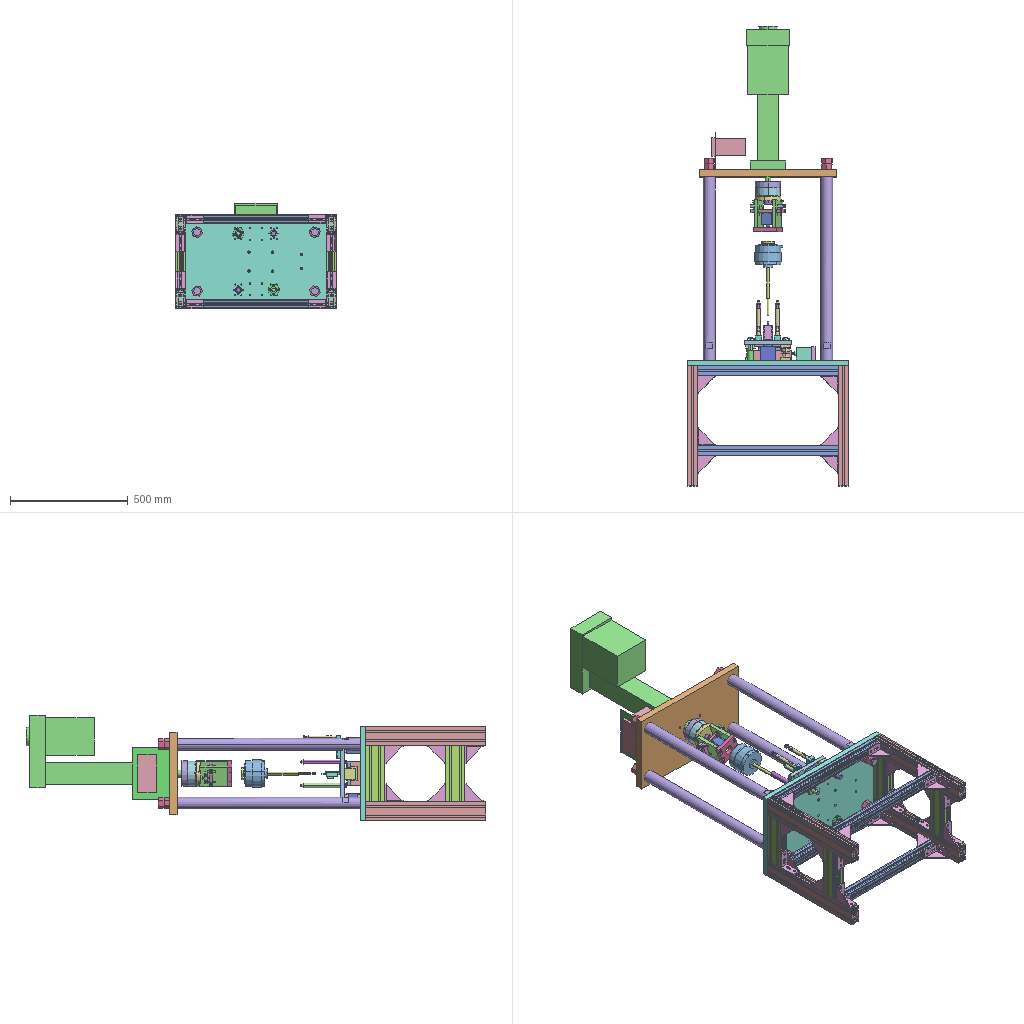Assembly | STEP file | 47 different items | 124 placed | box 680 x 1953 x 448 mm
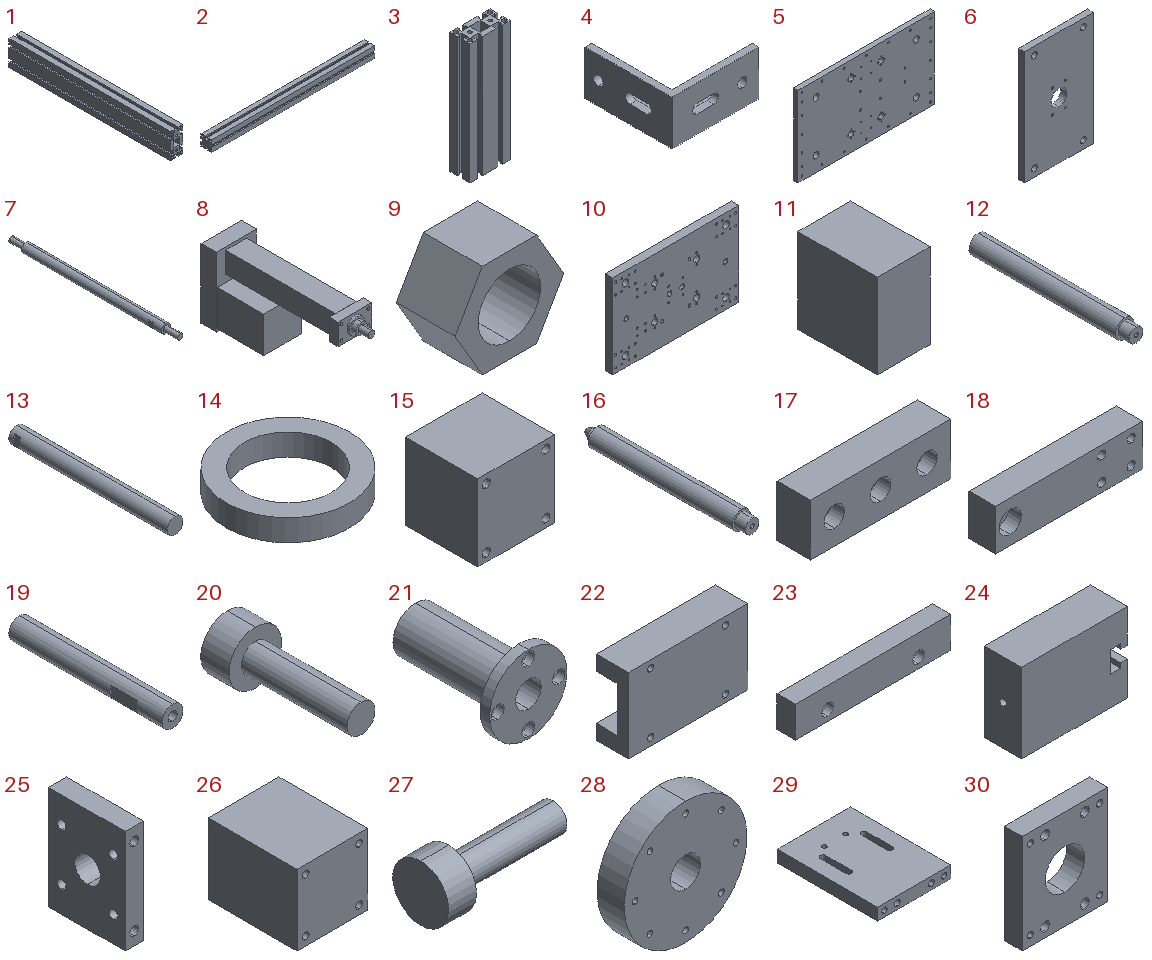Parts list (item | name | quantity | size | volume):
1 | - | x4 | 40 x 510 x 80 mm | 928333 mm3
2 | - | x4 | 600 x 40 x 40 mm | 535009 mm3
3 | - | x4 | 80 x 40 x 240 mm | 436902 mm3
4 | - | x24 | 78 x 78 x 40 mm | 44331 mm3
5 | - | x1 | 680 x 22 x 400 mm | 5788922 mm3
6 | - | x1 | 350 x 30 x 580 mm | 5843358 mm3
7 | - | x4 | 50 x 940 x 50 mm | 1640944 mm3
8 | - | x1 | 180 x 686 x 308 mm | 14325025 mm3
9 | - | x16 | 46.188 x 25 x 40 mm | 20852 mm3
10 | - | x1 | 300 x 18 x 200 mm | 1023453 mm3
11 | - | x1 | 30 x 45 x 48 mm | 61923 mm3
12 | - | x2 | 20 x 170 x 20 mm | 51580 mm3
13 | - | x2 | 16 x 160 x 16 mm | 31996 mm3
14 | - | x8 | 17 x 17 x 3 mm | 341.648 mm3
15 | - | x2 | 64 x 68.5 x 64 mm | 240094 mm3
16 | - | x2 | 20 x 181 x 20 mm | 52508 mm3
17 | - | x4 | 38 x 9 x 14 mm | 3259 mm3
18 | - | x2 | 100 x 18 x 28 mm | 45388 mm3
19 | - | x2 | 16 x 117 x 16 mm | 21831 mm3
20 | - | x2 | 15 x 38 x 15 mm | 2735 mm3
21 | - | x2 | 48 x 70 x 48 mm | 35205 mm3
22 | - | x1 | 160 x 43 x 100 mm | 410478 mm3
23 | - | x2 | 120 x 14 x 24 mm | 36593 mm3
24 | - | x1 | 80 x 28 x 60 mm | 129360 mm3
25 | - | x1 | 14 x 59 x 80 mm | 56725 mm3
26 | - | x1 | 53 x 73.5 x 53 mm | 182241 mm3
27 | - | x1 | 38 x 16 x 16 mm | 3116 mm3
28 | - | x1 | 108 x 24 x 108 mm | 204189 mm3
29 | - | x2 | 86 x 118 x 14 mm | 130717 mm3
30 | - | x1 | 86 x 18 x 100 mm | 121674 mm3
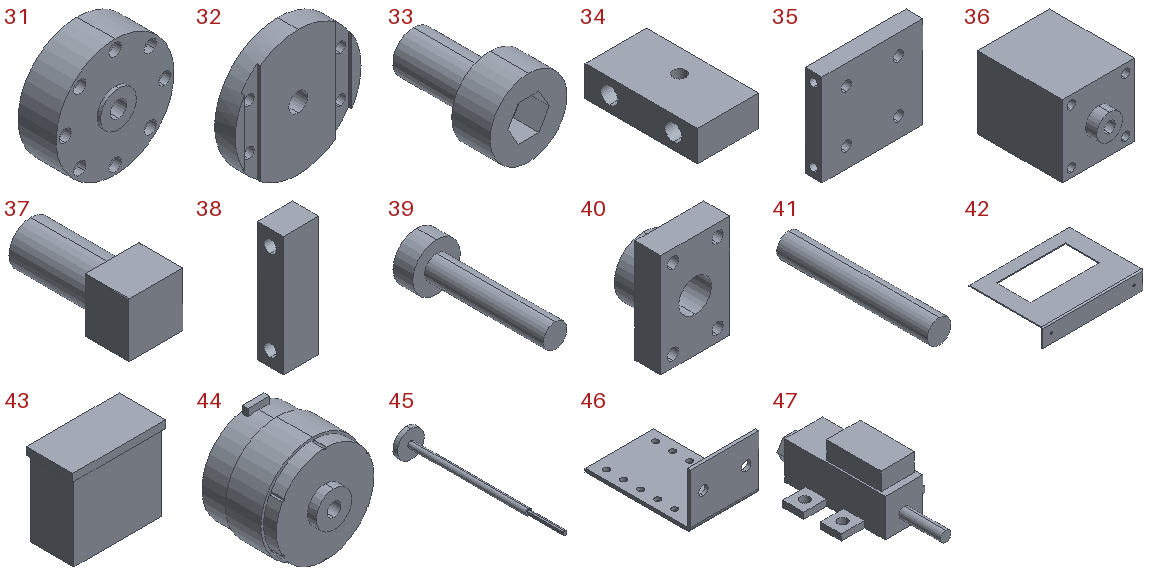31 | NS-TH3B-3t | x1 | 105 x 37 x 105 mm | 278290 mm3
32 | - | x1 | 110 x 18 x 110 mm | 153241 mm3
33 | M16X1.5 screw | x1 | 30 x 45 x 30 mm | 14937 mm3
34 | - | x2 | 24 x 44 x 12 mm | 10016 mm3
35 | - | x1 | 66 x 11 x 60 mm | 39291 mm3
36 | - | x1 | 45 x 60 x 45 mm | 101884 mm3
37 | - | x1 | 10 x 23 x 10 mm | 1554 mm3
38 | - | x2 | 19 x 14 x 64 mm | 14945 mm3
39 | - | x2 | 12 x 35 x 12 mm | 1414 mm3
40 | - | x4 | 40 x 30 x 60 mm | 39122 mm3
41 | - | x2 | 19 x 120 x 19 mm | 34023 mm3
42 | - | x1 | 220 x 160 x 40 mm | 64047 mm3
43 | NS-YB05C-A1 (five-digit digital display, with 232 interface) | x1 | 160 x 80 x 143 mm | 1638650 mm3
44 | - | x1 | 116 x 98 x 120 mm | 586421 mm3
45 | - | x1 | 53 x 313.9 x 53 mm | 49554 mm3
46 | - | x1 | 40 x 62 x 32 mm | 7034 mm3
47 | NS-WY02-10 | x1 | 40 x 75 x 26.6 mm | 21245 mm3
Placements (level | parent | child | x y z in mm | rotation matrix by rows):
1 | subassembly 2 | subassembly 3 | 787.547 322.833 225.0 | 1 0 0 0 1 0 0 0 1
2 | subassembly 3 | subassembly 4 | -13.187 -523.467 -0.0 | 1 0 0 0 1 0 0 0 1
2 | subassembly 3 | subassembly 5 | -633.187 -33.467 20.0 | 1 0 0 0 0 -1 0 1 0
2 | subassembly 3 | subassembly 4 | -653.187 -523.467 -0.0 | 1 0 0 0 1 0 0 0 1
2 | subassembly 3 | subassembly 6 | -13.187 -53.467 -280.0 | 0 1 0 -1 0 0 0 0 1
2 | subassembly 3 | subassembly 4 | -13.187 -523.467 -320.0 | 1 0 0 0 1 0 0 0 1
2 | subassembly 3 | subassembly 5 | -633.187 -33.467 -340.0 | 1 0 0 0 0 -1 0 1 0
2 | subassembly 3 | subassembly 4 | -653.187 -523.467 -320.0 | 1 0 0 0 1 0 0 0 1
2 | subassembly 3 | subassembly 6 | -653.187 -53.467 -280.0 | 0 1 0 -1 0 0 0 0 1
2 | subassembly 3 | subassembly 5 | -633.187 -373.467 20.0 | 1 0 0 0 0 -1 0 1 0
2 | subassembly 3 | subassembly 5 | -633.187 -373.467 -340.0 | 1 0 0 0 0 1 0 -1 0
2 | subassembly 3 | subassembly 6 | -13.187 -393.467 -280.0 | 0 1 0 -1 0 0 0 0 1
2 | subassembly 3 | subassembly 6 | -653.187 -393.467 -280.0 | 0 -1 0 1 0 0 0 0 1
2 | subassembly 3 | subassembly 7 | -633.187 -353.467 20.0 | 1 0 0 0 1 0 0 0 1
2 | subassembly 3 | subassembly 7 | -633.187 -353.467 -340.0 | 1 0 0 0 1 0 0 0 1
2 | subassembly 3 | subassembly 7 | -33.187 -353.467 -340.0 | -1 0 0 0 1 0 0 0 -1
2 | subassembly 3 | subassembly 7 | -33.187 -353.467 20.0 | -1 0 0 0 1 0 0 0 -1
2 | subassembly 3 | subassembly 7 | -33.187 -53.467 20.0 | -1 0 0 0 -1 0 0 0 1
2 | subassembly 3 | subassembly 7 | -33.187 -53.467 -340.0 | -1 0 0 0 -1 0 0 0 1
2 | subassembly 3 | subassembly 7 | -633.187 -53.467 -340.0 | 1 0 0 0 -1 0 0 0 -1
2 | subassembly 3 | subassembly 7 | -633.187 -53.467 20.0 | 1 0 0 0 -1 0 0 0 -1
2 | subassembly 3 | subassembly 7 | -653.187 -353.467 -40.0 | 0 0 1 0 1 0 -1 0 0
2 | subassembly 3 | subassembly 7 | -653.187 -353.467 -280.0 | 0 0 1 1 0 0 0 1 -0
2 | subassembly 3 | subassembly 7 | -653.187 -93.467 -280.0 | 0 0 -1 -1 0 0 0 1 -0
2 | subassembly 3 | subassembly 7 | -653.187 -93.467 -40.0 | 0 0 1 -1 0 0 0 -1 -0
2 | subassembly 3 | subassembly 7 | -13.187 -93.467 -40.0 | 0 0 1 -1 0 0 0 -1 -0
2 | subassembly 3 | subassembly 7 | -13.187 -93.467 -280.0 | 0 0 -1 -1 0 0 0 1 -0
2 | subassembly 3 | subassembly 7 | -13.187 -353.467 -40.0 | 0 0 1 0 1 0 -1 0 0
2 | subassembly 3 | subassembly 7 | -13.187 -353.467 -280.0 | 0 0 -1 0 1 0 1 0 -0
2 | subassembly 3 | subassembly 7 | -13.187 -433.467 -40.0 | 0 0 -1 0 -1 0 -1 0 0
2 | subassembly 3 | subassembly 7 | -13.187 -433.467 -280.0 | 0 0 1 0 -1 0 1 0 0
2 | subassembly 3 | subassembly 7 | -33.187 -393.467 -340.0 | -1 0 0 0 -1 0 0 0 1
2 | subassembly 3 | subassembly 7 | -633.187 -393.467 -340.0 | 0 1 0 -1 0 0 0 0 1
2 | subassembly 3 | subassembly 7 | -33.187 -393.467 20.0 | -1 0 0 0 -1 0 0 0 1
2 | subassembly 3 | subassembly 7 | -633.187 -393.467 20.0 | 1 0 0 0 -1 0 0 0 -1
2 | subassembly 3 | subassembly 7 | -653.187 -433.467 -40.0 | 0 0 -1 0 -1 0 -1 0 0
2 | subassembly 3 | subassembly 7 | -653.187 -433.467 -280.0 | 0 0 1 0 -1 0 1 0 -0
1 | subassembly 2 | subassembly 8 | 454.36 309.366 65.0 | 1 0 0 0 1 0 0 0 1
1 | subassembly 2 | subassembly 9 | 454.36 1142.927 90.761 | 0 0 -1 0 1 0 1 0 -0
2 | subassembly 9 | subassembly 10 | -25.761 -31.561 -0.0 | 1 0 0 0 1 0 0 0 1
2 | subassembly 9 | subassembly 11 | -150.761 -891.561 250.0 | -0.6182 0 0.7861 0 1 0 -0.7861 0 -0.6182
2 | subassembly 9 | subassembly 11 | 99.239 -891.561 250.0 | 1 0 0 0 1 0 0 0 1
2 | subassembly 9 | subassembly 11 | 99.239 -891.561 -250.0 | 1 0 0 0 1 0 0 0 1
2 | subassembly 9 | subassembly 11 | -150.761 -891.561 -250.0 | 1 0 0 0 1 0 0 0 1
2 | subassembly 9 | subassembly 12 | -25.761 -1.56 -0.0 | 0 0 -1 0 1 0 1 0 0
2 | subassembly 9 | subassembly 13 | -150.761 -1.56 250.0 | 1 0 0 0 1 0 0 0 1
2 | subassembly 9 | subassembly 13 | -150.761 23.439 250.0 | 0.9957 0 -0.09229 0 1 0 0.09229 0 0.9957
2 | subassembly 9 | subassembly 13 | 99.239 -1.56 250.0 | 0.9957 0 -0.09229 0 1 0 0.09229 0 0.9957
2 | subassembly 9 | subassembly 13 | 99.239 23.439 250.0 | 0.9957 0 -0.09229 0 1 0 0.09229 0 0.9957
2 | subassembly 9 | subassembly 13 | 99.239 -1.56 -250.0 | 0.9957 0 -0.09229 0 1 0 0.09229 0 0.9957
2 | subassembly 9 | subassembly 13 | 99.239 23.439 -250.0 | 0.9836 0 -0.1802 0 1 0 0.1802 0 0.9836
2 | subassembly 9 | subassembly 13 | -150.761 -1.56 -250.0 | 0.9836 0 -0.1802 0 1 0 0.1802 0 0.9836
2 | subassembly 9 | subassembly 13 | -150.761 23.439 -250.0 | 0.9626 0 -0.2709 0 1 0 0.2709 0 0.9626
1 | subassembly 2 | subassembly 14 | 454.36 412.776 36.213 | 0 0 1 0 1 0 -1 0 0
2 | subassembly 14 | subassembly 15 | -28.787 -12.909 -0.0 | 1 0 0 0 1 0 0 0 1
2 | subassembly 14 | subassembly 16 | -28.787 -57.909 -0.0 | 0 0 -1 0 1 0 1 0 0
2 | subassembly 14 | subassembly 17 | -78.787 -6.909 -40.0 | 1 0 0 0 1 0 0 0 1
2 | subassembly 14 | subassembly 17 | 21.213 -6.909 40.0 | 1 0 0 0 1 0 0 0 1
2 | subassembly 14 | subassembly 18 | 91.213 -144.909 75.0 | 0 0 -1 0 1 0 1 0 0
2 | subassembly 14 | subassembly 18 | -148.787 -144.909 -75.0 | 0 0 -1 0 1 0 1 0 0
2 | subassembly 14 | subassembly 19 | 91.213 5.091 62.0 | 1 0 0 0 1 0 0 0 1
2 | subassembly 14 | subassembly 19 | 91.213 5.091 88.0 | 1 0 0 0 1 0 0 0 1
2 | subassembly 14 | subassembly 20 | 89.213 -81.409 0.0 | 1 0 0 0 1 0 0 0 1
2 | subassembly 14 | subassembly 20 | -146.787 -81.409 0.0 | 0.9989 0 -0.04696 0 1 0 0.04696 0 0.9989
2 | subassembly 14 | subassembly 19 | 91.213 5.091 -88.0 | 1 0 0 0 1 0 0 0 1
2 | subassembly 14 | subassembly 19 | 91.213 5.091 -62.0 | 1 0 0 0 1 0 0 0 1
2 | subassembly 14 | subassembly 19 | -148.787 5.091 88.0 | 1 0 0 0 1 0 0 0 1
2 | subassembly 14 | subassembly 19 | -148.787 5.091 62.0 | 1 0 0 0 1 0 0 0 1
2 | subassembly 14 | subassembly 19 | -148.787 5.091 -88.0 | 1 0 0 0 1 0 0 0 1
2 | subassembly 14 | subassembly 19 | -148.787 5.091 -62.0 | 1 0 0 0 1 0 0 0 1
2 | subassembly 14 | subassembly 21 | -78.787 -6.909 40.0 | 1 0 0 0 1 0 0 0 1
2 | subassembly 14 | subassembly 21 | 21.213 -6.909 -40.0 | 1 0 0 0 1 0 0 0 1
2 | subassembly 14 | subassembly 22 | 21.213 -12.909 40.0 | 0 0 -1 0 -1 0 -1 0 0
2 | subassembly 14 | subassembly 22 | -78.787 -12.909 40.0 | 0 0 -1 0 -1 0 -1 0 0
2 | subassembly 14 | subassembly 22 | -78.787 -12.909 -40.0 | 0 0 -1 0 -1 0 -1 0 0
2 | subassembly 14 | subassembly 22 | 21.213 -12.909 -40.0 | 0 0 -1 0 -1 0 -1 0 0
2 | subassembly 14 | subassembly 23 | 28.48 -1.675 -80.0 | 1 0 0 0 1 0 0 0 1
3 | subassembly 23 | subassembly 24 | -121.267 6.766 40.0 | 1 0 0 0 1 0 0 0 1
3 | subassembly 23 | subassembly 25 | -211.267 24.766 40.0 | 1 0 0 0 1 0 0 0 1
3 | subassembly 23 | subassembly 26 | -211.267 126.766 40.0 | 0.9997 0 0.02485 0 1 0 -0.02485 0 0.9997
2 | subassembly 14 | subassembly 23 | 28.48 -1.675 -0.0 | 1 0 0 0 1 0 0 0 1
3 | subassembly 23 | subassembly 24 | -121.267 6.766 40.0 | 1 0 0 0 1 0 0 0 1
3 | subassembly 23 | subassembly 25 | -211.267 24.766 40.0 | 1 0 0 0 1 0 0 0 1
3 | subassembly 23 | subassembly 26 | -211.267 126.766 40.0 | 0.9997 0 0.02485 0 1 0 -0.02485 0 0.9997
1 | subassembly 2 | subassembly 27 | 529.36 303.366 -55.0 | 1 0 0 0 1 0 0 0 1
1 | subassembly 2 | subassembly 27 | 379.36 303.366 185.0 | 0.3234 0 0.9462 0 1 0 -0.9462 0 0.3234
1 | subassembly 2 | subassembly 13 | 704.36 284.366 -60.0 | 0.3024 0 0.9532 0 1 0 -0.9532 0 0.3024
1 | subassembly 2 | subassembly 13 | 704.36 259.366 -60.0 | 0.3024 0 0.9532 0 1 0 -0.9532 0 0.3024
1 | subassembly 2 | subassembly 13 | 704.36 284.366 190.0 | 0.1617 0 0.9868 0 1 0 -0.9868 0 0.1617
1 | subassembly 2 | subassembly 13 | 704.36 259.366 190.0 | 0.6487 0 0.7611 0 1 0 -0.7611 0 0.6487
1 | subassembly 2 | subassembly 13 | 204.359 284.366 190.0 | 0.8809 0 0.4733 0 1 0 -0.4733 0 0.8809
1 | subassembly 2 | subassembly 13 | 204.359 259.366 190.0 | 0.9802 0 0.1978 0 1 0 -0.1978 0 0.9802
1 | subassembly 2 | subassembly 13 | 204.359 284.366 -60.0 | 0.9885 0 0.151 0 1 0 -0.151 0 0.9885
1 | subassembly 2 | subassembly 13 | 204.359 259.366 -60.0 | 0.9885 0 0.151 0 1 0 -0.151 0 0.9885
1 | subassembly 2 | subassembly 28 | 528.87 353.051 65.0 | 1 0 0 0 1 0 0 0 1
2 | subassembly 28 | subassembly 29 | -54.511 -21.684 -0.0 | 1 0 0 0 1 0 0 0 1
2 | subassembly 28 | subassembly 30 | -54.511 21.316 -50.0 | 1 0 0 0 1 0 0 0 1
2 | subassembly 28 | subassembly 30 | -54.511 21.316 50.0 | -1 0 0 0 1 0 0 0 -1
2 | subassembly 28 | subassembly 31 | -15.011 -6.684 0.0 | 1 0 0 0 1 0 0 0 1
2 | subassembly 28 | subassembly 32 | 157.076 10.163 0.0 | 1 0 0 0 1 0 0 0 1
3 | subassembly 32 | subassembly 33 | -38.586 -31.847 -0.0 | 1 0 0 0 1 0 0 0 1
3 | subassembly 32 | subassembly 34 | -45.586 -2.847 -0.0 | 0 -1 0 1 0 0 0 0 1
3 | subassembly 32 | subassembly 35 | -107.086 -2.847 -0.0 | 1 0 0 0 1 0 0 0 1
1 | subassembly 2 | subassembly 36 | 430.954 1071.539 66.021 | 0.999 0 0.04358 0 1 0 -0.04358 0 0.999
2 | subassembly 36 | subassembly 37 | 23.427 -5.172 -0.0 | 1 0 0 0 1 0 0 0 1
2 | subassembly 36 | subassembly 38 | -14.35 -175.172 -13.149 | -0.3287 0 -0.9444 0 1 0 0.9444 0 -0.3287
2 | subassembly 36 | subassembly 38 | 61.205 -175.172 13.149 | -0.3287 0 -0.9444 0 1 0 0.9444 0 -0.3287
2 | subassembly 36 | subassembly 39 | 23.427 -175.172 0.0 | 0.3287 0 -0.9444 0 -1 0 -0.9444 0 -0.3287
2 | subassembly 36 | NS-TH3B-3t | 23.427 -5.172 -0.0 | 1 0 0 0 1 0 0 0 1
2 | subassembly 36 | subassembly 40 | 23.427 -60.172 0.0 | -0.9444 0 0.3287 0 1 0 -0.3287 0 -0.9444
2 | subassembly 36 | M16X1.5 screw | 23.427 -75.172 -0.0 | 1 0 0 0 1 0 0 0 1
2 | subassembly 36 | subassembly 41 | -20.961 -82.172 -15.45 | -0.9444 -0.3287 0 0 0 1 -0.3287 0.9444 0
2 | subassembly 36 | subassembly 42 | 7.33 -113.425 -5.603 | 0.9444 0 -0.3287 0 1 0 0.3287 0 0.9444
3 | subassembly 42 | subassembly 43 | 17.045 8.753 -0.0 | 1 0 0 0 1 0 0 0 1
3 | subassembly 42 | subassembly 44 | 17.045 -49.747 -0.0 | 1 0 0 0 1 0 0 0 1
3 | subassembly 42 | subassembly 45 | 17.045 -64.747 -0.0 | 1 0 0 0 1 0 0 0 1
2 | subassembly 36 | subassembly 46 | 67.816 -104.672 15.45 | 0.9444 0 -0.3287 0 1 0 0.3287 0 0.9444
2 | subassembly 36 | subassembly 46 | -20.961 -104.672 -15.45 | -0.9444 0 0.3287 0 1 0 -0.3287 0 -0.9444
2 | subassembly 36 | subassembly 41 | 67.816 -82.172 15.45 | 0.9444 0.3287 0 0 0 1 0.3287 -0.9444 0
2 | subassembly 36 | subassembly 47 | 81.982 -95.872 20.38 | 0.116 0 0.9933 0 1 0 -0.9933 0 0.116
2 | subassembly 36 | subassembly 47 | -35.127 -96.457 -20.38 | 0.116 0 0.9933 0 1 0 -0.9933 0 0.116
1 | subassembly 2 | subassembly 48 | 508.629 389.934 185.0 | -1 0 0 0 -1 0 0 0 1
2 | subassembly 48 | subassembly 49 | -20.73 -9.933 0.0 | 1 0 0 0 1 0 0 0 1
2 | subassembly 48 | subassembly 50 | -20.73 -9.933 0.0 | 0.9575 0 0.2884 0 1 0 -0.2884 0 0.9575
1 | subassembly 2 | subassembly 49 | 529.36 331.366 185.0 | -1 0 0 0 1 0 0 0 -1
1 | subassembly 2 | subassembly 48 | 358.629 389.934 -55.0 | -1 0 0 0 -1 0 0 0 1
2 | subassembly 48 | subassembly 49 | -20.73 -9.933 0.0 | 1 0 0 0 1 0 0 0 1
2 | subassembly 48 | subassembly 50 | -20.73 -9.933 0.0 | 0.9575 0 0.2884 0 1 0 -0.2884 0 0.9575
1 | subassembly 2 | subassembly 49 | 379.36 331.366 -55.0 | -1 0 0 0 1 0 0 0 -1
1 | subassembly 2 | subassembly 51 | 244.359 1222.441 124.992 | 0 0 -1 0 1 0 1 0 -0
2 | subassembly 51 | subassembly 52 | -169.992 -81.075 15.0 | 1 0 0 0 1 0 0 0 1
2 | subassembly 51 | NS-YB05C-A1 (five-digit digital display, with 232 interface) | -59.992 16.425 15.0 | 1 0 0 0 1 0 0 0 1
1 | subassembly 2 | subassembly 53 | 452.705 769.876 43.684 | -0.1703 0 0.9854 0 1 0 -0.9854 0 -0.1703
2 | subassembly 53 | subassembly 54 | -21.286 -42.11 -2.0 | 1 0 0 0 1 0 0 0 1
2 | subassembly 53 | subassembly 55 | -21.286 -245.41 -2.0 | -0.9481 0 0.3179 0 1 0 -0.3179 0 -0.9481
1 | subassembly 2 | subassembly 56 | 478.161 445.642 88.0 | 1 0 0 0 1 0 0 0 1
2 | subassembly 56 | subassembly 57 | -23.801 -25.775 -14.0 | 1 0 0 0 1 0 0 0 1
2 | subassembly 56 | NS-WY02-10 | -23.801 30.225 -16.0 | 1 0 0 0 -1 0 0 0 -1